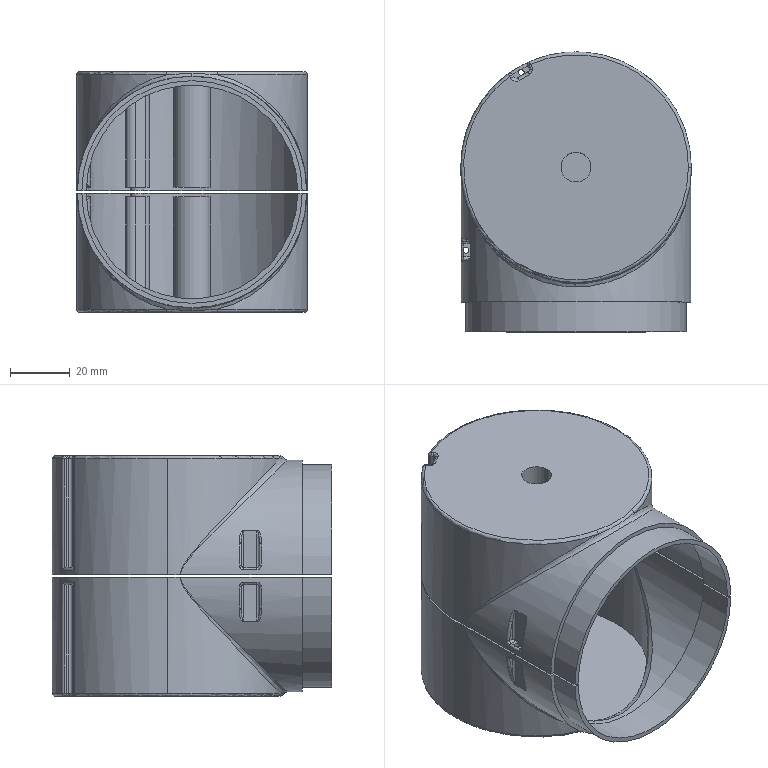Part | SolidWorks | features ICE 7, Fillet 4, Extrusion 1, MirrorSolid 1, Scale 1, Shell 1 | 2 solids | 180 faces | box 77.5 x 94 x 80.75 mm | volume 41607 mm3 | cylinder 86 | plane 58 | torus 18 | spline 14 | sphere 4 | commonest cylinder face diameters 2 x24 1.5 x12 4.5 x12 4 x8 75 x6 77.5 x6